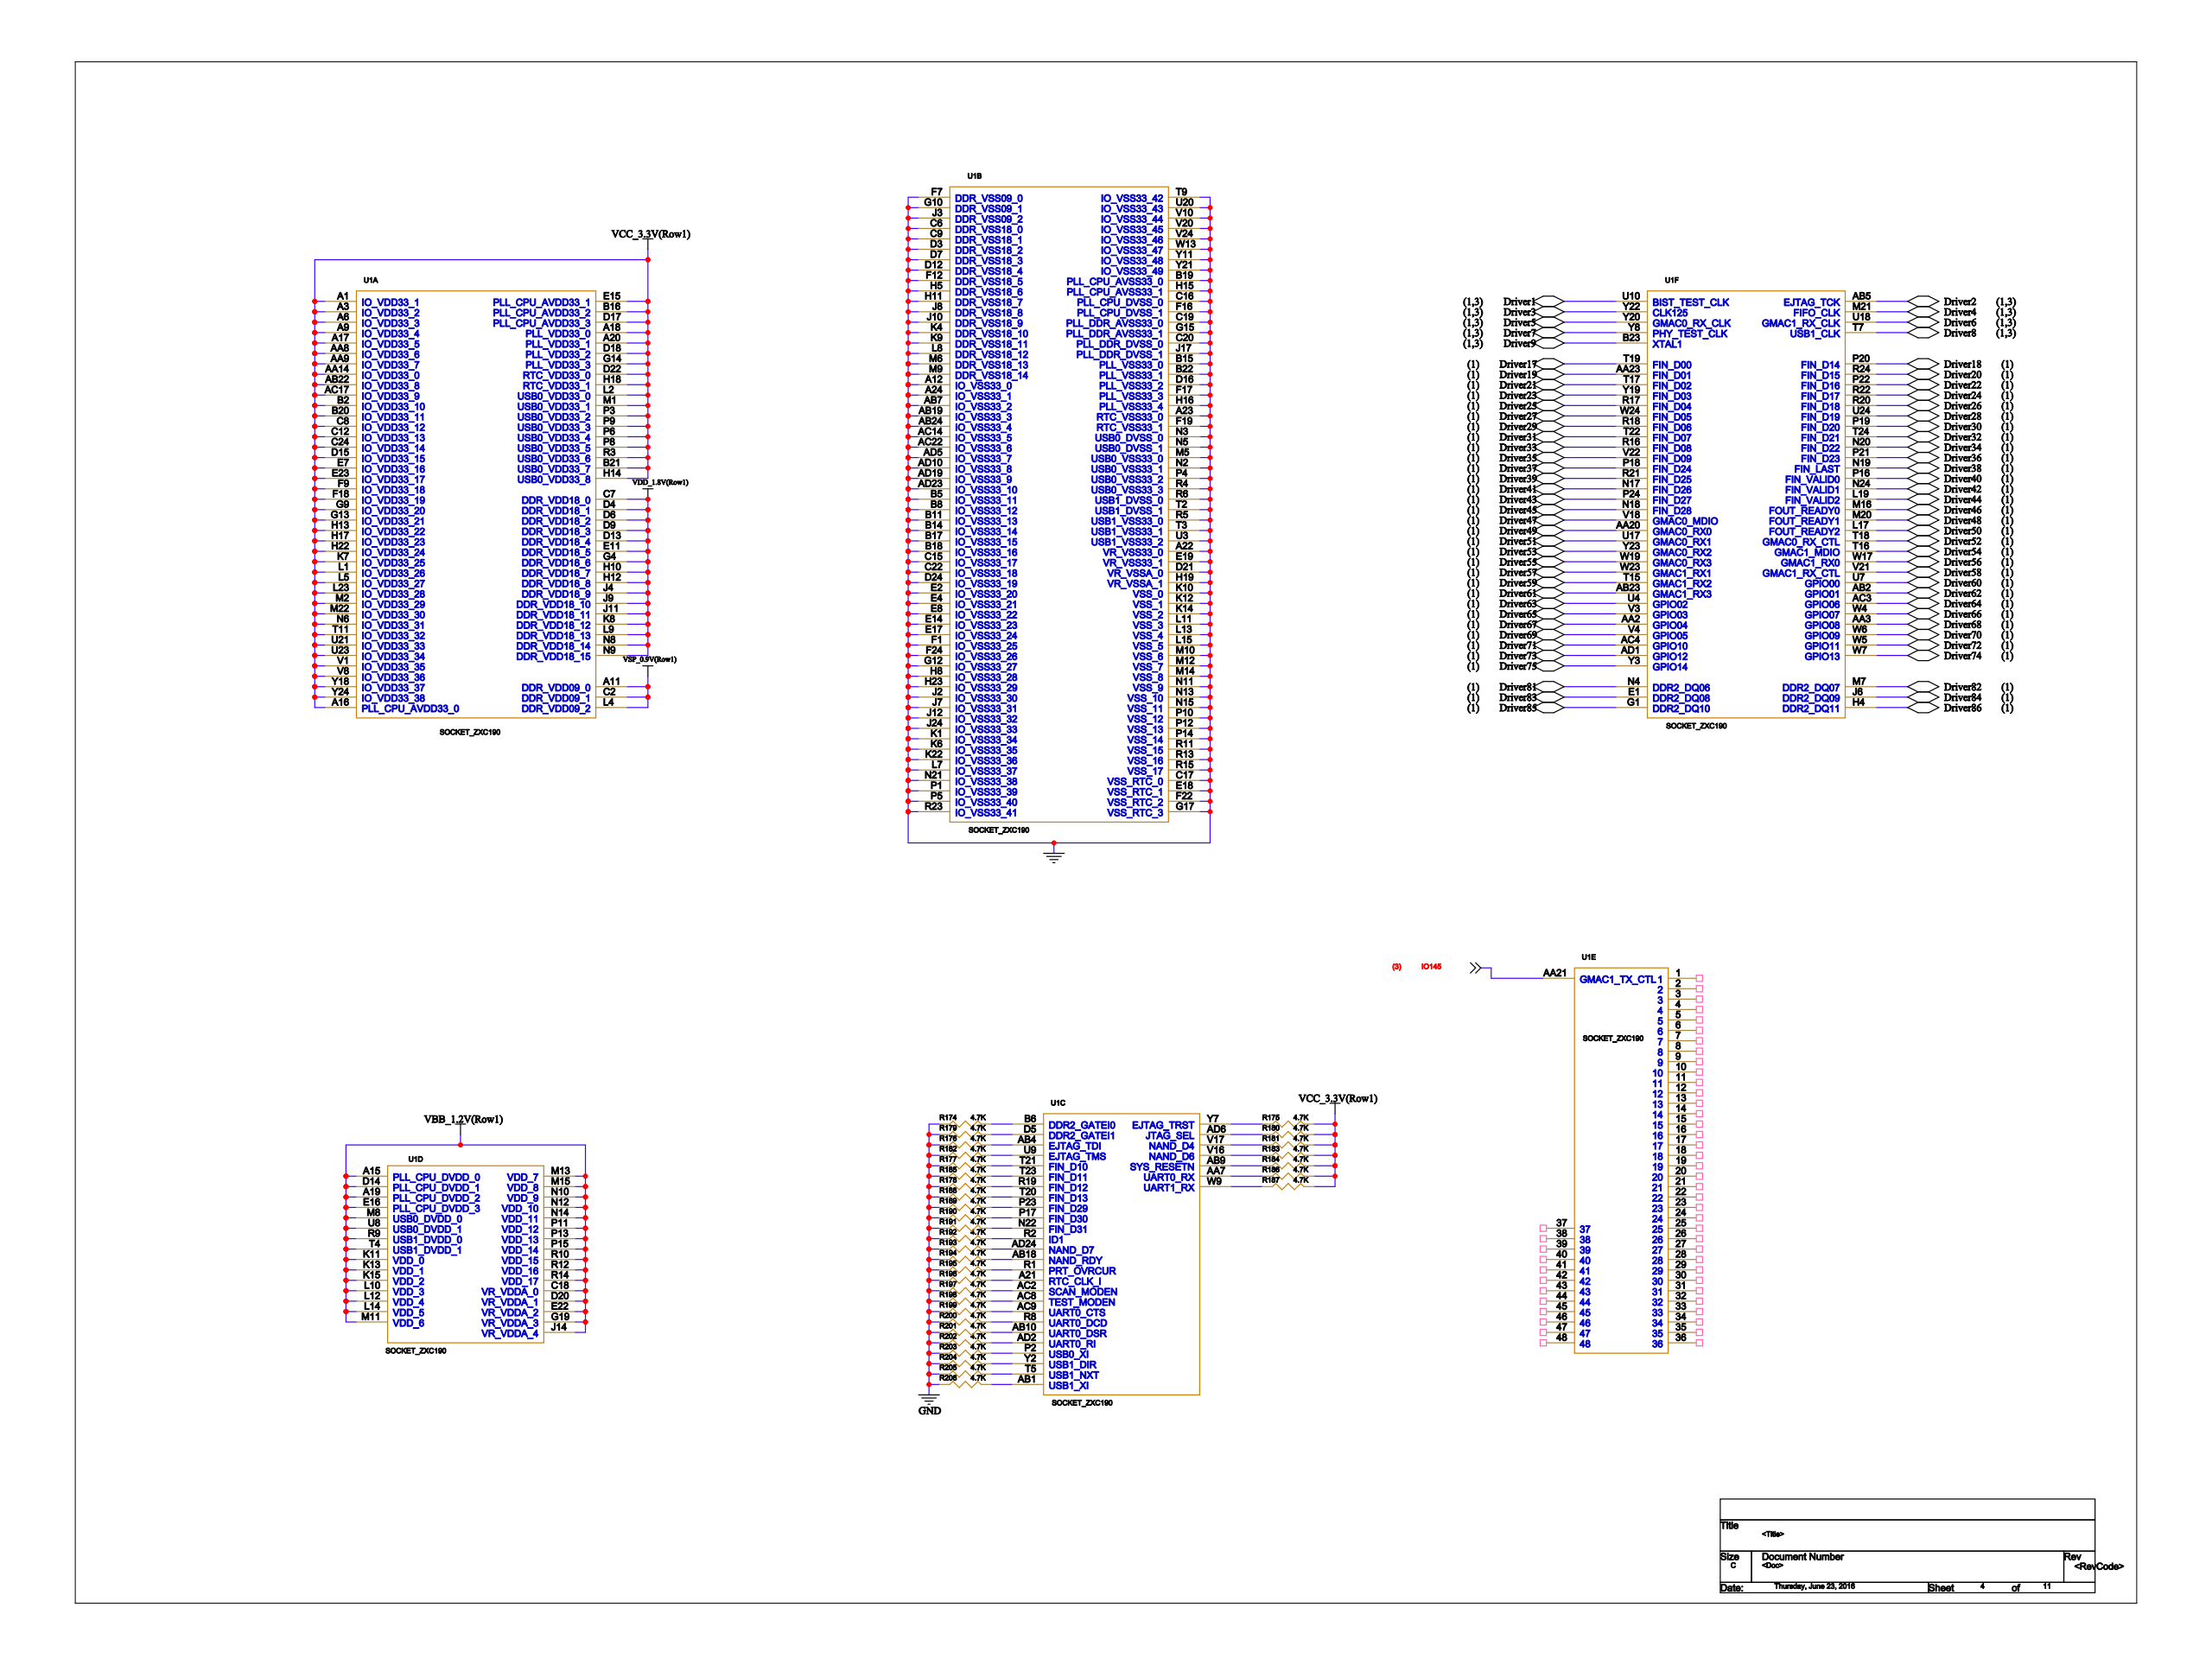Circuit board | Cadence Allegro | 531 parts | 624 nets | one sheet of the schematic
Parts on this sheet (reference | value | footprint):
R174 | 4.7K | R0805
R175 | 4.7K | R0805
R176 | 4.7K | R0805
R177 | 4.7K | R0805
R178 | 4.7K | R0805
R179 | 4.7K | R0805
R180 | 4.7K | R0805
R181 | 4.7K | R0805
R182 | 4.7K | R0805
R183 | 4.7K | R0805
R184 | 4.7K | R0805
R185 | 4.7K | R0805
R186 | 4.7K | R0805
R187 | 4.7K | R0805
R188 | 4.7K | R0805
R189 | 4.7K | R0805
R190 | 4.7K | R0805
R191 | 4.7K | R0805
R192 | 4.7K | R0805
R193 | 4.7K | R0805
R194 | 4.7K | R0805
R195 | 4.7K | R0805
R196 | 4.7K | R0805
R197 | 4.7K | R0805
R198 | 4.7K | R0805
R199 | 4.7K | R0805
R200 | 4.7K | R0805
R201 | 4.7K | R0805
R202 | 4.7K | R0805
R203 | 4.7K | R0805
R204 | 4.7K | R0805
R205 | 4.7K | R0805
R206 | 4.7K | R0805
U1 | SOCKET_ZXC190 | BGA-576
U3 | SOCKET_ZXC190 | BGA-576
U4 | SOCKET_ZXC190 | BGA-576
U10 | SOCKET_ZXC190 | BGA-576
Nets of these parts (net: part-pin ...):
GND: R174-1 R176-1 R177-1 R178-1 R179-1 R182-1 R185-1 R188-1 R189-1 R190-1 R191-1 R192-1 R193-1 R194-1 R195-1 R196-1 R197-1 R198-1 R199-1 R200-1 R201-1 R202-1 R203-1 R204-1 R205-1 R206-1 U1-A12 U1-A22 U1-A23 U1-A24 U1-AB7 U1-AB19 U1-AB24 U1-AC14 U1-AC22 U1-AD5 U1-AD10 U1-AD19 U1-AD23 U1-B5 U1-B8 U1-B11 U1-B14 U1-B15 U1-B17 U1-B18 U1-B19 U1-B22 U1-C6 U1-C9 U1-C15 U1-C16 U1-C17 U1-C19 U1-C20 U1-C22 U1-D3 U1-D7 U1-D12 U1-D16 U1-D21 U1-D24 U1-E2 U1-E4 U1-E8 U1-E14 U1-E17 U1-E18 U1-E19 U1-F1 U1-F7 U1-F12 U1-F16 U1-F17 U1-F19 U1-F22 U1-F24 U1-G10 U1-G12 U1-G15 U1-G17 U1-H5 U1-H8 U1-H11 U1-H15 U1-H16 U1-H19 U1-H23 U1-J2 U1-J3 U1-J7 U1-J8 U1-J10 U1-J12 U1-J17 U1-J24 U1-K1 U1-K4 U1-K6 U1-K9 U1-K10 U1-K12 U1-K14 U1-K22 U1-L7 U1-L8 U1-L11 U1-L13 U1-L15 U1-M5 U1-M6 U1-M9 U1-M10 U1-M12 U1-M14 U1-N2 U1-N3 U1-N5 U1-N11 U1-N13 U1-N15 U1-N21 U1-P1 U1-P4 U1-P5 U1-P10 U1-P12 U1-P14 U1-R4 U1-R5 U1-R6 U1-R11 U1-R13 U1-R15 U1-R23 U1-T2 U1-T3 U1-T9 U1-U3 U1-U20 U1-V10 U1-V20 U1-V24 U1-W13 U1-Y11 U1-Y21 U3-A12 U3-A22 U3-A23 U3-A24 U3-AB7 U3-AB19 U3-AB24 U3-AC14 U3-AC22 U3-AD5 U3-AD10 U3-AD19 U3-AD23 U3-B5 U3-B8 U3-B11 U3-B14 U3-B15 U3-B17 U3-B18 U3-B19 U3-B22 U3-C6 U3-C9 U3-C15 U3-C16 U3-C17 U3-C19 U3-C20 U3-C22 U3-D3 U3-D7 U3-D12 U3-D16 U3-D21 U3-D24 U3-E2 U3-E4 U3-E8 U3-E14 U3-E17 U3-E18 U3-E19 U3-F1 U3-F7 U3-F12 U3-F16 U3-F17 U3-F19 U3-F22 U3-F24 U3-G10 U3-G12 U3-G15 U3-G17 U3-H5 U3-H8 U3-H11 U3-H15 U3-H16 U3-H19 U3-H23 U3-J2 U3-J3 U3-J7 U3-J8 U3-J10 U3-J12 U3-J17 U3-J24 U3-K1 U3-K4 U3-K6 U3-K9 U3-K10 U3-K12 U3-K14 U3-K22 U3-L7 U3-L8 U3-L11 U3-L13 U3-L15 U3-M5 U3-M6 U3-M9 U3-M10 U3-M12 U3-M14 U3-N2 U3-N3 U3-N5 U3-N11 U3-N13 U3-N15 U3-N21 U3-P1 U3-P4 U3-P5 U3-P10 U3-P12 U3-P14 U3-R4 U3-R5 U3-R6 U3-R11 U3-R13 U3-R15 U3-R23 U3-T2 U3-T3 U3-T9 U3-U3 U3-U20 U3-V10 U3-V20 U3-V24 U3-W13 U3-Y11 U3-Y21 U4-A12 U4-A22 U4-A23 U4-A24 U4-AB7 U4-AB19 U4-AB24 U4-AC14 U4-AC22 U4-AD5 U4-AD10 U4-AD19 U4-AD23 U4-B5 U4-B8 U4-B11 U4-B14 U4-B15 U4-B17 U4-B18 U4-B19 U4-B22 U4-C6 U4-C9 U4-C15 U4-C16 U4-C17 U4-C19 U4-C20 U4-C22 U4-D3 U4-D7 U4-D12 U4-D16 U4-D21 U4-D24 U4-E2 U4-E4 U4-E8 U4-E14 U4-E17 U4-E18 U4-E19 U4-F1 U4-F7 U4-F12 U4-F16 U4-F17 U4-F19 U4-F22 U4-F24 U4-G10 U4-G12 U4-G15 U4-G17 U4-H5 U4-H8 U4-H11 U4-H15 U4-H16 U4-H19 U4-H23 U4-J2 U4-J3 U4-J7 U4-J8 U4-J10 U4-J12 U4-J17 U4-J24 U4-K1 U4-K4 U4-K6 U4-K9 U4-K10 U4-K12 U4-K14 U4-K22 U4-L7 U4-L8 U4-L11 U4-L13 U4-L15 U4-M5 U4-M6 U4-M9 U4-M10 U4-M12 U4-M14 U4-N2 U4-N3 U4-N5 U4-N11 U4-N13 U4-N15 U4-N21 U4-P1 U4-P4 U4-P5 U4-P10 U4-P12 U4-P14 U4-R4 U4-R5 U4-R6 U4-R11 U4-R13 U4-R15 U4-R23 U4-T2 U4-T3 U4-T9 U4-U3 U4-U20 U4-V10 U4-V20 U4-V24 U4-W13 U4-Y11 U4-Y21 U10-A12 U10-A22 U10-A23 U10-A24 U10-AB7 U10-AB19 U10-AB24 U10-AC14 U10-AC22 U10-AD5 U10-AD10 U10-AD19 U10-AD23 U10-B5 U10-B8 U10-B11 U10-B14 U10-B15 U10-B17 U10-B18 U10-B19 U10-B22 U10-C6 U10-C9 U10-C15 U10-C16 U10-C17 U10-C19 U10-C20 U10-C22 U10-D3 U10-D7 U10-D12 U10-D16 U10-D21 U10-D24 U10-E2 U10-E4 U10-E8 U10-E14 U10-E17 U10-E18 U10-E19 U10-F1 U10-F7 U10-F12 U10-F16 U10-F17 U10-F19 U10-F22 U10-F24 U10-G10 U10-G12 U10-G15 U10-G17 U10-H5 U10-H8 U10-H11 U10-H15 U10-H16 U10-H19 U10-H23 U10-J2 U10-J3 U10-J7 U10-J8 U10-J10 U10-J12 U10-J17 U10-J24 U10-K1 U10-K4 U10-K6 U10-K9 U10-K10 U10-K12 U10-K14 U10-K22 U10-L7 U10-L8 U10-L11 U10-L13 U10-L15 U10-M5 U10-M6 U10-M9 U10-M10 U10-M12 U10-M14 U10-N2 U10-N3 U10-N5 U10-N11 U10-N13 U10-N15 U10-N21 U10-P1 U10-P4 U10-P5 U10-P10 U10-P12 U10-P14 U10-R4 U10-R5 U10-R6 U10-R11 U10-R13 U10-R15 U10-R23 U10-T2 U10-T3 U10-T9 U10-U3 U10-U20 U10-V10 U10-V20 U10-V24 U10-W13 U10-Y11 U10-Y21
N15507: R174-2 U1-B6
N43793: R175-1 U1-Y7
VCC_3.3V(ROW1): R175-2 R180-2 R181-2 R183-2 R184-2 R186-2 R187-2 U1-A1 U1-A3 U1-A6 U1-A9 U1-A16 U1-A17 U1-A18 U1-A20 U1-AA8 U1-AA9 U1-AA14 U1-AB22 U1-AC17 U1-B2 U1-B16 U1-B20 U1-B21 U1-C8 U1-C12 U1-C24 U1-D15 U1-D17 U1-D18 U1-D22 U1-E7 U1-E15 U1-E23 U1-F9 U1-F18 U1-G9 U1-G13 U1-G14 U1-H13 U1-H14 U1-H17 U1-H18 U1-H22 U1-K7 U1-L1 U1-L2 U1-L5 U1-L23 U1-M1 U1-M2 U1-M22 U1-N6 U1-P3 U1-P6 U1-P8 U1-P9 U1-R3 U1-T11 U1-U21 U1-U23 U1-V1 U1-V8 U1-Y18 U1-Y24 U3-A1 U3-A3 U3-A6 U3-A9 U3-A16 U3-A17 U3-A18 U3-A20 U3-AA8 U3-AA9 U3-AA14 U3-AB22 U3-AC17 U3-B2 U3-B16 U3-B20 U3-B21 U3-C8 U3-C12 U3-C24 U3-D15 U3-D17 U3-D18 U3-D22 U3-E7 U3-E15 U3-E23 U3-F9 U3-F18 U3-G9 U3-G13 U3-G14 U3-H13 U3-H14 U3-H17 U3-H18 U3-H22 U3-K7 U3-L1 U3-L2 U3-L5 U3-L23 U3-M1 U3-M2 U3-M22 U3-N6 U3-P3 U3-P6 U3-P8 U3-P9 U3-R3 U3-T11 U3-U21 U3-U23 U3-V1 U3-V8 U3-Y18 U3-Y24 U4-A1 U4-A3 U4-A6 U4-A9 U4-A16 U4-A17 U4-A18 U4-A20 U4-AA8 U4-AA9 U4-AA14 U4-AB22 U4-AC17 U4-B2 U4-B16 U4-B20 U4-B21 U4-C8 U4-C12 U4-C24 U4-D15 U4-D17 U4-D18 U4-D22 U4-E7 U4-E15 U4-E23 U4-F9 U4-F18 U4-G9 U4-G13 U4-G14 U4-H13 U4-H14 U4-H17 U4-H18 U4-H22 U4-K7 U4-L1 U4-L2 U4-L5 U4-L23 U4-M1 U4-M2 U4-M22 U4-N6 U4-P3 U4-P6 U4-P8 U4-P9 U4-R3 U4-T11 U4-U21 U4-U23 U4-V1 U4-V8 U4-Y18 U4-Y24
N15511: R176-2 U1-AB4
N15515: R177-2 U1-T21
N15519: R178-2 U1-R19
N15509: R179-2 U1-D5
N31163: R180-1 U1-AD6
N37011: R181-1 U1-V17
N15513: R182-2 U1-U9
N37887: R183-1 U1-V16
N38765: R184-1 U1-AB9
N15517: R185-2 U1-T23
N8412852: R186-1 U1-AA7
N41283: R187-1 U1-W9
N15521: R188-2 U1-T20
N15523: R189-2 U1-P23
N15525: R190-2 U1-P17
N15527: R191-2 U1-N22
N15529: R192-2 U1-R2
N15531: R193-2 U1-AD24
N15533: R194-2 U1-AB18
N15535: R195-2 U1-R1
N15537: R196-2 U1-A21
N15539: R197-2 U1-AC2
N15541: R198-2 U1-AC8
N15543: R199-2 U1-AC9
N8423644: R200-2 U1-R8
N15547: R201-2 U1-AB10
N15549: R202-2 U1-AD2
N15551: R203-2 U1-P2
N15553: R204-2 U1-Y2
N15555: R205-2 U1-T5
N15557: R206-2 U1-AB1
IO145: U1-AA21